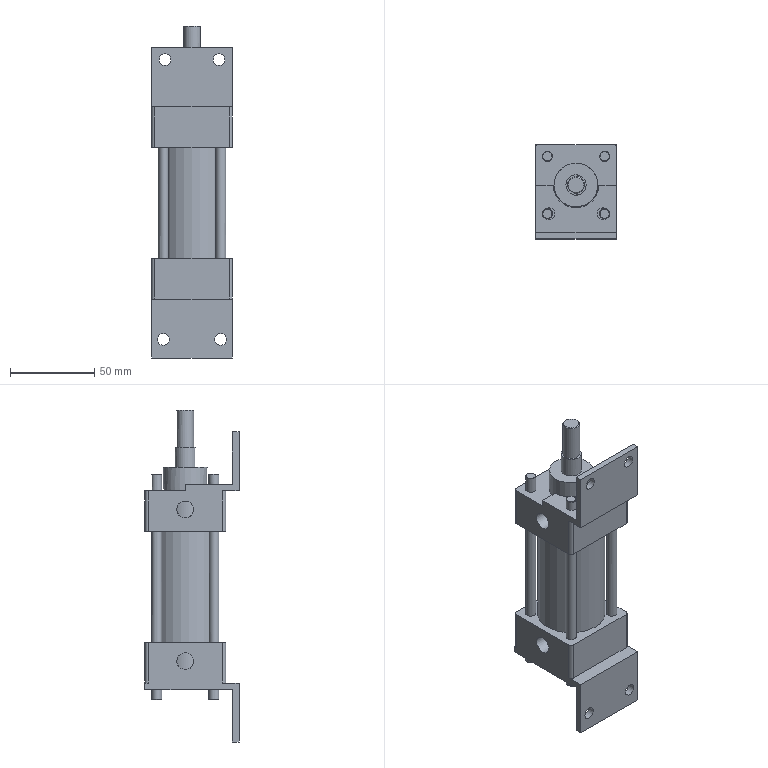Part | NX | features solid 2 | 1 solid | 94 faces | box 48 x 56 x 197 mm | volume 219893 mm3 | plane 44 | cylinder 41 | cone 9 | commonest cylinder face diameters 6 x12 7 x10 4 x8 26 x4 10 x3 12 x1